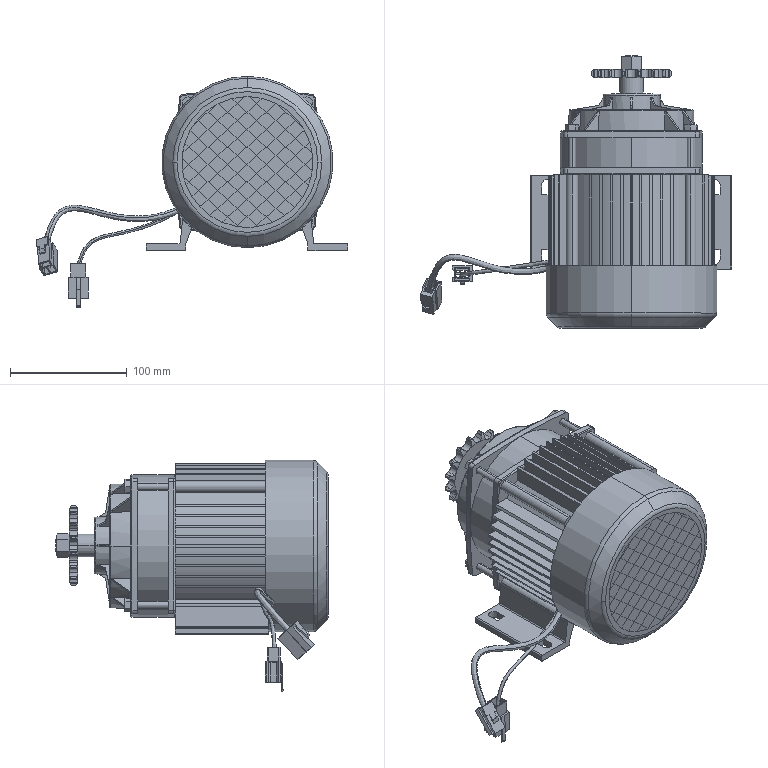Part | SolidWorks | 6 solids | 849 faces | box 267.158 x 234 x 198.451 mm | volume 1799732 mm3 | plane 502 | cylinder 242 | torus 58 | cone 42 | spline 5 | commonest cylinder face diameters 121 x36 142.263 x34 12.473 x32 22.269 x32 8.653 x21 70 x16